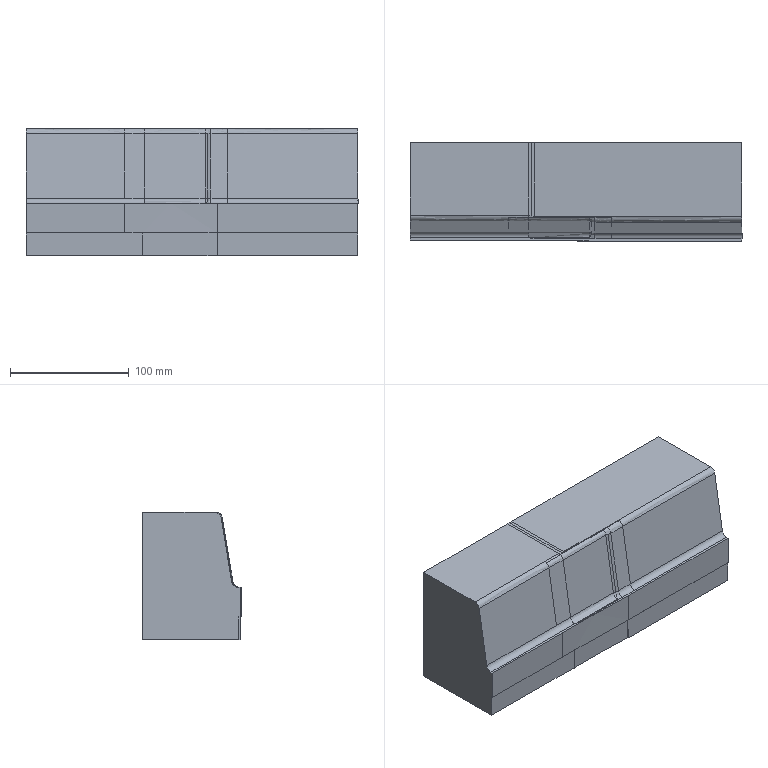Part | NX | features solid 2 | 1 solid | 55 faces | box 280 x 83.171 x 107.133 mm | volume 2238545 mm3 | spline 25 | plane 20 | cylinder 7 | cone 3 | commonest cylinder face diameters 12 x3 10 x2 20 x2